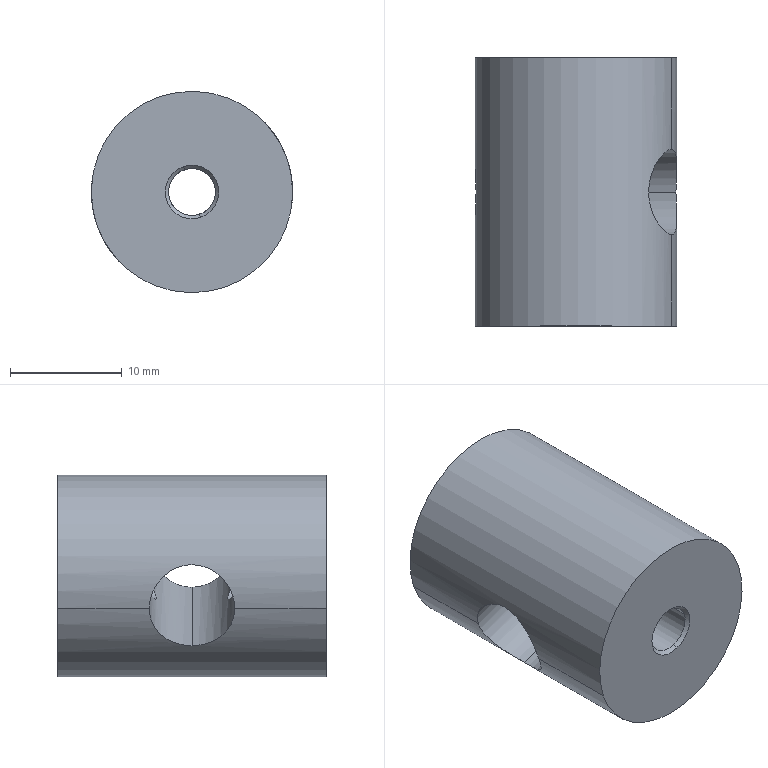Part | STEP file | 2026.6.15-Main Assembly图.sldasm-Part-182 | 1 solid | 14 faces | box 18 x 24 x 18 mm | volume 5067 mm3 | cylinder 8 | cone 4 | plane 2 | commonest cylinder face diameters 4.2 x4 7.65 x2 18 x2
STEP:
#1=CARTESIAN_POINT('',(-1463.721,1436.264,3252.695));
#2=VERTEX_POINT('',#1);
#3=CARTESIAN_POINT('',(-1463.437,1435.964,3252.791));
#4=VERTEX_POINT('',#3);
#5=CARTESIAN_POINT('',(-1463.721,1436.264,3252.695));
#6=DIRECTION('',(0.6699,-0.7071,0.2262));
#7=VECTOR('',#6,1000.);
#8=LINE('',#5,#7);
#9=EDGE_CURVE('',#2,#4,#8,.T.);
#10=ORIENTED_EDGE('',*,*,#9,.T.);
#11=CARTESIAN_POINT('',(-1459.458,1435.964,3254.134));
#12=VERTEX_POINT('',#11);
#13=CARTESIAN_POINT('',(-1461.448,1435.964,3253.462));
#14=DIRECTION('',(0.,-1.,0.));
#15=DIRECTION('',(0.9474,0.,0.3199));
#16=AXIS2_PLACEMENT_3D('',#13,#14,#15);
#17=CIRCLE('',#16,2.1);
#18=EDGE_CURVE('',#4,#12,#17,.T.);
#19=ORIENTED_EDGE('',*,*,#18,.T.);
#20=CARTESIAN_POINT('',(-1459.174,1436.264,3254.23));
#21=VERTEX_POINT('',#20);
#22=CARTESIAN_POINT('',(-1459.174,1436.264,3254.23));
#23=DIRECTION('',(-0.6699,-0.7071,-0.2262));
#24=VECTOR('',#23,1000.);
#25=LINE('',#22,#24);
#26=EDGE_CURVE('',#21,#12,#25,.T.);
#27=ORIENTED_EDGE('',*,*,#26,.F.);
#28=CARTESIAN_POINT('',(-1461.448,1436.264,3253.462));
#29=DIRECTION('',(0.,-1.,0.));
#30=DIRECTION('',(0.9474,0.,0.3199));
#31=AXIS2_PLACEMENT_3D('',#28,#29,#30);
#32=CIRCLE('',#31,2.4);
#33=EDGE_CURVE('',#2,#21,#32,.T.);
#34=ORIENTED_EDGE('',*,*,#33,.F.);
#35=EDGE_LOOP('',(#10,#19,#27,#34));
#36=FACE_OUTER_BOUND('',#35,.T.);
#37=CARTESIAN_POINT('',(-1461.448,1436.264,3253.462));
#38=DIRECTION('',(0.,1.,0.));
#39=DIRECTION('',(-0.9474,0.,-0.3199));
#40=AXIS2_PLACEMENT_3D('',#37,#38,#39);
#41=CONICAL_SURFACE('',#40,2.4,0.7854);
#42=ADVANCED_FACE('',(#36),#41,.F.);
#43=CARTESIAN_POINT('',(-1462.12,1412.564,3255.452));
#44=VERTEX_POINT('',#43);
#45=CARTESIAN_POINT('',(-1462.216,1412.264,3255.736));
#46=VERTEX_POINT('',#45);
#47=CARTESIAN_POINT('',(-1462.216,1412.264,3255.736));
#48=DIRECTION('',(-0.2262,-0.7071,0.6699));
#49=VECTOR('',#48,1000.);
#50=LINE('',#47,#49);
#51=EDGE_CURVE('',#44,#46,#50,.T.);
#52=ORIENTED_EDGE('',*,*,#51,.F.);
#53=CARTESIAN_POINT('',(-1459.458,1412.564,3254.134));
#54=VERTEX_POINT('',#53);
#55=CARTESIAN_POINT('',(-1461.448,1412.564,3253.462));
#56=DIRECTION('',(0.,1.,0.));
#57=DIRECTION('',(0.9474,0.,0.3199));
#58=AXIS2_PLACEMENT_3D('',#55,#56,#57);
#59=CIRCLE('',#58,2.1);
#60=EDGE_CURVE('',#44,#54,#59,.T.);
#61=ORIENTED_EDGE('',*,*,#60,.T.);
#62=CARTESIAN_POINT('',(-1460.776,1412.564,3251.473));
#63=VERTEX_POINT('',#62);
#64=CARTESIAN_POINT('',(-1461.448,1412.564,3253.462));
#65=DIRECTION('',(0.,1.,0.));
#66=DIRECTION('',(0.9474,0.,0.3199));
#67=AXIS2_PLACEMENT_3D('',#64,#65,#66);
#68=CIRCLE('',#67,2.1);
#69=EDGE_CURVE('',#54,#63,#68,.T.);
#70=ORIENTED_EDGE('',*,*,#69,.T.);
#71=CARTESIAN_POINT('',(-1460.68,1412.264,3251.189));
#72=VERTEX_POINT('',#71);
#73=CARTESIAN_POINT('',(-1460.68,1412.264,3251.189));
#74=DIRECTION('',(0.2262,-0.7071,-0.6699));
#75=VECTOR('',#74,1000.);
#76=LINE('',#73,#75);
#77=EDGE_CURVE('',#63,#72,#76,.T.);
#78=ORIENTED_EDGE('',*,*,#77,.T.);
#79=CARTESIAN_POINT('',(-1461.448,1412.264,3253.462));
#80=DIRECTION('',(0.,-1.,0.));
#81=DIRECTION('',(0.3199,0.,-0.9474));
#82=AXIS2_PLACEMENT_3D('',#79,#80,#81);
#83=CIRCLE('',#82,2.4);
#84=EDGE_CURVE('',#72,#46,#83,.T.);
#85=ORIENTED_EDGE('',*,*,#84,.T.);
#86=EDGE_LOOP('',(#52,#61,#70,#78,#85));
#87=FACE_OUTER_BOUND('',#86,.T.);
#88=CARTESIAN_POINT('',(-1461.448,1412.264,3253.462));
#89=DIRECTION('',(0.,-1.,0.));
#90=DIRECTION('',(-0.3199,0.,0.9474));
#91=AXIS2_PLACEMENT_3D('',#88,#89,#90);
#92=CONICAL_SURFACE('',#91,2.4,0.7854);
#93=ADVANCED_FACE('',(#87),#92,.F.);
#94=CARTESIAN_POINT('',(-1463.437,1420.439,3252.791));
#95=VERTEX_POINT('',#94);
#96=CARTESIAN_POINT('',(-1463.437,1412.564,3252.791));
#97=VERTEX_POINT('',#96);
#98=CARTESIAN_POINT('',(-1463.437,1436.264,3252.791));
#99=DIRECTION('',(0.,-1.,0.));
#100=VECTOR('',#99,1000.);
#101=LINE('',#98,#100);
#102=EDGE_CURVE('',#95,#97,#101,.T.);
#103=ORIENTED_EDGE('',*,*,#102,.T.);
#104=CARTESIAN_POINT('',(-1461.448,1412.564,3253.462));
#105=DIRECTION('',(0.,1.,0.));
#106=DIRECTION('',(0.9474,0.,0.3199));
#107=AXIS2_PLACEMENT_3D('',#104,#105,#106);
#108=CIRCLE('',#107,2.1);
#109=EDGE_CURVE('',#63,#97,#108,.T.);
#110=ORIENTED_EDGE('',*,*,#109,.F.);
#111=ORIENTED_EDGE('',*,*,#69,.F.);
#112=CARTESIAN_POINT('',(-1459.458,1420.439,3254.134));
#113=VERTEX_POINT('',#112);
#114=CARTESIAN_POINT('',(-1459.458,1436.264,3254.134));
#115=DIRECTION('',(0.,-1.,0.));
#116=VECTOR('',#115,1000.);
#117=LINE('',#114,#116);
#118=EDGE_CURVE('',#113,#54,#117,.T.);
#119=ORIENTED_EDGE('',*,*,#118,.F.);
#120=CARTESIAN_POINT('',(-1459.458,1420.439,3254.134));
#121=CARTESIAN_POINT('',(-1459.413,1420.439,3254.));
#122=CARTESIAN_POINT('',(-1459.382,1420.447,3253.864));
#123=CARTESIAN_POINT('',(-1459.347,1420.477,3253.588));
#124=CARTESIAN_POINT('',(-1459.343,1420.5,3253.447));
#125=CARTESIAN_POINT('',(-1459.373,1420.582,3253.035));
#126=CARTESIAN_POINT('',(-1459.447,1420.66,3252.769));
#127=CARTESIAN_POINT('',(-1459.626,1420.78,3252.408));
#128=CARTESIAN_POINT('',(-1459.698,1420.821,3252.293));
#129=CARTESIAN_POINT('',(-1459.863,1420.898,3252.078));
#130=CARTESIAN_POINT('',(-1459.954,1420.934,3251.98));
#131=CARTESIAN_POINT('',(-1460.158,1420.996,3251.799));
#132=CARTESIAN_POINT('',(-1460.272,1421.022,3251.717));
#133=CARTESIAN_POINT('',(-1460.512,1421.058,3251.577));
#134=CARTESIAN_POINT('',(-1460.639,1421.067,3251.519));
#135=CARTESIAN_POINT('',(-1460.904,1421.068,3251.429));
#136=CARTESIAN_POINT('',(-1461.044,1421.058,3251.397));
#137=CARTESIAN_POINT('',(-1461.319,1421.023,3251.362));
#138=CARTESIAN_POINT('',(-1461.459,1420.997,3251.358));
#139=CARTESIAN_POINT('',(-1461.87,1420.904,3251.387));
#140=CARTESIAN_POINT('',(-1462.135,1420.82,3251.46));
#141=CARTESIAN_POINT('',(-1462.617,1420.66,3251.697));
#142=CARTESIAN_POINT('',(-1462.838,1420.583,3251.865));
#143=CARTESIAN_POINT('',(-1463.11,1420.5,3252.172));
#144=CARTESIAN_POINT('',(-1463.193,1420.478,3252.286));
#145=CARTESIAN_POINT('',(-1463.334,1420.447,3252.528));
#146=CARTESIAN_POINT('',(-1463.392,1420.439,3252.656));
#147=CARTESIAN_POINT('',(-1463.437,1420.439,3252.791));
#148=B_SPLINE_CURVE_WITH_KNOTS('',3,(#120,#121,#122,#123,#124,#125,#126,#127,#128,#129,#130,#131,#132,#133,#134,#135,#136,#137,#138,#139,#140,#141,#142,#143,#144,#145,#146,#147),.UNSPECIFIED.,.F.,.F.,(4,2,2,2,2,2,2,2,2,2,2,2,2,4),(0.,0.000419,0.000838,0.001676,0.002095,0.002514,0.002933,0.003352,0.003771,0.00419,0.005028,0.005866,0.006285,0.006704),.UNSPECIFIED.);
#149=EDGE_CURVE('',#113,#95,#148,.T.);
#150=ORIENTED_EDGE('',*,*,#149,.T.);
#151=EDGE_LOOP('',(#103,#110,#111,#119,#150));
#152=FACE_OUTER_BOUND('',#151,.T.);
#153=CARTESIAN_POINT('',(-1461.448,1436.264,3253.462));
#154=DIRECTION('',(0.,1.,0.));
#155=DIRECTION('',(-0.9474,0.,-0.3199));
#156=AXIS2_PLACEMENT_3D('',#153,#154,#155);
#157=CYLINDRICAL_SURFACE('',#156,2.1);
#158=ADVANCED_FACE('',(#152),#157,.F.);
#159=CARTESIAN_POINT('',(-1463.437,1428.089,3252.791));
#160=VERTEX_POINT('',#159);
#161=CARTESIAN_POINT('',(-1463.437,1436.264,3252.791));
#162=DIRECTION('',(0.,-1.,0.));
#163=VECTOR('',#162,1000.);
#164=LINE('',#161,#163);
#165=EDGE_CURVE('',#4,#160,#164,.T.);
#166=ORIENTED_EDGE('',*,*,#165,.T.);
#167=CARTESIAN_POINT('',(-1459.458,1428.089,3254.134));
#168=VERTEX_POINT('',#167);
#169=CARTESIAN_POINT('',(-1463.437,1428.089,3252.791));
#170=CARTESIAN_POINT('',(-1463.392,1428.089,3252.656));
#171=CARTESIAN_POINT('',(-1463.334,1428.081,3252.529));
#172=CARTESIAN_POINT('',(-1463.194,1428.052,3252.289));
#173=CARTESIAN_POINT('',(-1463.112,1428.029,3252.174));
#174=CARTESIAN_POINT('',(-1462.838,1427.946,3251.865));
#175=CARTESIAN_POINT('',(-1462.618,1427.869,3251.698));
#176=CARTESIAN_POINT('',(-1462.257,1427.749,3251.52));
#177=CARTESIAN_POINT('',(-1462.13,1427.708,3251.472));
#178=CARTESIAN_POINT('',(-1461.869,1427.63,3251.401));
#179=CARTESIAN_POINT('',(-1461.736,1427.594,3251.378));
#180=CARTESIAN_POINT('',(-1461.465,1427.532,3251.358));
#181=CARTESIAN_POINT('',(-1461.324,1427.506,3251.362));
#182=CARTESIAN_POINT('',(-1461.048,1427.471,3251.396));
#183=CARTESIAN_POINT('',(-1460.913,1427.461,3251.427));
#184=CARTESIAN_POINT('',(-1460.647,1427.461,3251.516));
#185=CARTESIAN_POINT('',(-1460.517,1427.471,3251.575));
#186=CARTESIAN_POINT('',(-1460.276,1427.506,3251.714));
#187=CARTESIAN_POINT('',(-1460.163,1427.531,3251.796));
#188=CARTESIAN_POINT('',(-1459.853,1427.625,3252.068));
#189=CARTESIAN_POINT('',(-1459.687,1427.708,3252.287));
#190=CARTESIAN_POINT('',(-1459.448,1427.868,3252.768));
#191=CARTESIAN_POINT('',(-1459.374,1427.946,3253.035));
#192=CARTESIAN_POINT('',(-1459.343,1428.029,3253.444));
#193=CARTESIAN_POINT('',(-1459.347,1428.051,3253.585));
#194=CARTESIAN_POINT('',(-1459.381,1428.081,3253.863));
#195=CARTESIAN_POINT('',(-1459.413,1428.089,3254.));
#196=CARTESIAN_POINT('',(-1459.458,1428.089,3254.134));
#197=B_SPLINE_CURVE_WITH_KNOTS('',3,(#169,#170,#171,#172,#173,#174,#175,#176,#177,#178,#179,#180,#181,#182,#183,#184,#185,#186,#187,#188,#189,#190,#191,#192,#193,#194,#195,#196),.UNSPECIFIED.,.F.,.F.,(4,2,2,2,2,2,2,2,2,2,2,2,2,4),(0.,0.000419,0.000838,0.001676,0.002095,0.002514,0.002933,0.003352,0.003771,0.00419,0.005028,0.005866,0.006285,0.006704),.UNSPECIFIED.);
#198=EDGE_CURVE('',#160,#168,#197,.T.);
#199=ORIENTED_EDGE('',*,*,#198,.T.);
#200=CARTESIAN_POINT('',(-1459.458,1436.264,3254.134));
#201=DIRECTION('',(0.,-1.,0.));
#202=VECTOR('',#201,1000.);
#203=LINE('',#200,#202);
#204=EDGE_CURVE('',#12,#168,#203,.T.);
#205=ORIENTED_EDGE('',*,*,#204,.F.);
#206=ORIENTED_EDGE('',*,*,#18,.F.);
#207=EDGE_LOOP('',(#166,#199,#205,#206));
#208=FACE_OUTER_BOUND('',#207,.T.);
#209=CARTESIAN_POINT('',(-1461.448,1436.264,3253.462));
#210=DIRECTION('',(0.,1.,0.));
#211=DIRECTION('',(-0.9474,0.,-0.3199));
#212=AXIS2_PLACEMENT_3D('',#209,#210,#211);
#213=CYLINDRICAL_SURFACE('',#212,2.1);
#214=ADVANCED_FACE('',(#208),#213,.F.);
#215=CARTESIAN_POINT('',(-1469.975,1436.264,3250.583));
#216=VERTEX_POINT('',#215);
#217=CARTESIAN_POINT('',(-1452.921,1436.264,3256.342));
#218=VERTEX_POINT('',#217);
#219=CARTESIAN_POINT('',(-1461.448,1436.264,3253.462));
#220=DIRECTION('',(0.,-1.,0.));
#221=DIRECTION('',(-0.9474,0.,-0.3199));
#222=AXIS2_PLACEMENT_3D('',#219,#220,#221);
#223=CIRCLE('',#222,9.);
#224=EDGE_CURVE('',#216,#218,#223,.T.);
#225=ORIENTED_EDGE('',*,*,#224,.F.);
#226=CARTESIAN_POINT('',(-1461.448,1436.264,3253.462));
#227=DIRECTION('',(0.,-1.,0.));
#228=DIRECTION('',(-0.9474,0.,-0.3199));
#229=AXIS2_PLACEMENT_3D('',#226,#227,#228);
#230=CIRCLE('',#229,9.);
#231=EDGE_CURVE('',#218,#216,#230,.T.);
#232=ORIENTED_EDGE('',*,*,#231,.F.);
#233=EDGE_LOOP('',(#225,#232));
#234=FACE_OUTER_BOUND('',#233,.T.);
#235=CARTESIAN_POINT('',(-1461.448,1436.264,3253.462));
#236=DIRECTION('',(0.,-1.,0.));
#237=DIRECTION('',(0.9474,0.,0.3199));
#238=AXIS2_PLACEMENT_3D('',#235,#236,#237);
#239=CIRCLE('',#238,2.4);
#240=EDGE_CURVE('',#21,#2,#239,.T.);
#241=ORIENTED_EDGE('',*,*,#240,.T.);
#242=ORIENTED_EDGE('',*,*,#33,.T.);
#243=EDGE_LOOP('',(#241,#242));
#244=FACE_BOUND('',#243,.T.);
#245=CARTESIAN_POINT('',(-1461.448,1436.264,3253.462));
#246=DIRECTION('',(0.,1.,0.));
#247=DIRECTION('',(1.,0.,0.));
#248=AXIS2_PLACEMENT_3D('',#245,#246,#247);
#249=PLANE('',#248);
#250=ADVANCED_FACE('',(#234,#244),#249,.T.);
#251=CARTESIAN_POINT('',(-1469.975,1412.264,3250.583));
#252=VERTEX_POINT('',#251);
#253=CARTESIAN_POINT('',(-1452.921,1412.264,3256.342));
#254=VERTEX_POINT('',#253);
#255=CARTESIAN_POINT('',(-1461.448,1412.264,3253.462));
#256=DIRECTION('',(0.,1.,0.));
#257=DIRECTION('',(-0.9474,0.,-0.3199));
#258=AXIS2_PLACEMENT_3D('',#255,#256,#257);
#259=CIRCLE('',#258,9.);
#260=EDGE_CURVE('',#252,#254,#259,.T.);
#261=ORIENTED_EDGE('',*,*,#260,.F.);
#262=CARTESIAN_POINT('',(-1461.448,1412.264,3253.462));
#263=DIRECTION('',(0.,1.,0.));
#264=DIRECTION('',(-0.9474,0.,-0.3199));
#265=AXIS2_PLACEMENT_3D('',#262,#263,#264);
#266=CIRCLE('',#265,9.);
#267=EDGE_CURVE('',#254,#252,#266,.T.);
#268=ORIENTED_EDGE('',*,*,#267,.F.);
#269=EDGE_LOOP('',(#261,#268));
#270=FACE_OUTER_BOUND('',#269,.T.);
#271=ORIENTED_EDGE('',*,*,#84,.F.);
#272=CARTESIAN_POINT('',(-1461.448,1412.264,3253.462));
#273=DIRECTION('',(0.,-1.,0.));
#274=DIRECTION('',(0.3199,0.,-0.9474));
#275=AXIS2_PLACEMENT_3D('',#272,#273,#274);
#276=CIRCLE('',#275,2.4);
#277=EDGE_CURVE('',#46,#72,#276,.T.);
#278=ORIENTED_EDGE('',*,*,#277,.F.);
#279=EDGE_LOOP('',(#271,#278));
#280=FACE_BOUND('',#279,.T.);
#281=CARTESIAN_POINT('',(-1461.448,1412.264,3253.462));
#282=DIRECTION('',(0.,1.,0.));
#283=DIRECTION('',(1.,0.,0.));
#284=AXIS2_PLACEMENT_3D('',#281,#282,#283);
#285=PLANE('',#284);
#286=ADVANCED_FACE('',(#270,#280),#285,.F.);
#287=CARTESIAN_POINT('',(-1470.39,1424.264,3254.48));
#288=VERTEX_POINT('',#287);
#289=CARTESIAN_POINT('',(-1454.953,1424.264,3259.693));
#290=VERTEX_POINT('',#289);
#291=CARTESIAN_POINT('',(-1498.2,1424.264,3245.088));
#292=DIRECTION('',(0.9474,0.,0.3199));
#293=VECTOR('',#292,1000.);
#294=LINE('',#291,#293);
#295=EDGE_CURVE('',#288,#290,#294,.T.);
#296=ORIENTED_EDGE('',*,*,#295,.F.);
#297=CARTESIAN_POINT('',(-1469.975,1428.089,3250.583));
#298=VERTEX_POINT('',#297);
#299=CARTESIAN_POINT('',(-1469.975,1428.089,3250.583));
#300=CARTESIAN_POINT('',(-1470.056,1428.089,3250.825));
#301=CARTESIAN_POINT('',(-1470.126,1428.064,3251.067));
#302=CARTESIAN_POINT('',(-1470.245,1427.965,3251.547));
#303=CARTESIAN_POINT('',(-1470.294,1427.89,3251.789));
#304=CARTESIAN_POINT('',(-1470.369,1427.697,3252.251));
#305=CARTESIAN_POINT('',(-1470.396,1427.579,3252.472));
#306=CARTESIAN_POINT('',(-1470.432,1427.302,3252.896));
#307=CARTESIAN_POINT('',(-1470.442,1427.142,3253.097));
#308=CARTESIAN_POINT('',(-1470.449,1426.794,3253.462));
#309=CARTESIAN_POINT('',(-1470.447,1426.603,3253.629));
#310=CARTESIAN_POINT('',(-1470.437,1426.188,3253.926));
#311=CARTESIAN_POINT('',(-1470.429,1425.97,3254.053));
#312=CARTESIAN_POINT('',(-1470.413,1425.512,3254.26));
#313=CARTESIAN_POINT('',(-1470.405,1425.268,3254.343));
#314=CARTESIAN_POINT('',(-1470.393,1424.772,3254.452));
#315=CARTESIAN_POINT('',(-1470.39,1424.52,3254.48));
#316=CARTESIAN_POINT('',(-1470.39,1424.264,3254.48));
#317=B_SPLINE_CURVE_WITH_KNOTS('',3,(#299,#300,#301,#302,#303,#304,#305,#306,#307,#308,#309,#310,#311,#312,#313,#314,#315,#316),.UNSPECIFIED.,.F.,.F.,(4,2,2,2,2,2,2,2,4),(0.,0.0007561,0.001512,0.002268,0.003024,0.003781,0.004537,0.005293,0.006049),.UNSPECIFIED.);
#318=EDGE_CURVE('',#298,#288,#317,.T.);
#319=ORIENTED_EDGE('',*,*,#318,.F.);
#320=CARTESIAN_POINT('',(-1467.942,1424.264,3247.232));
#321=VERTEX_POINT('',#320);
#322=CARTESIAN_POINT('',(-1467.942,1424.264,3247.232));
#323=CARTESIAN_POINT('',(-1467.942,1424.52,3247.232));
#324=CARTESIAN_POINT('',(-1467.962,1424.771,3247.252));
#325=CARTESIAN_POINT('',(-1468.037,1425.264,3247.331));
#326=CARTESIAN_POINT('',(-1468.093,1425.508,3247.392));
#327=CARTESIAN_POINT('',(-1468.232,1425.969,3247.548));
#328=CARTESIAN_POINT('',(-1468.315,1426.188,3247.644));
#329=CARTESIAN_POINT('',(-1468.503,1426.601,3247.873));
#330=CARTESIAN_POINT('',(-1468.607,1426.794,3248.005));
#331=CARTESIAN_POINT('',(-1468.822,1427.142,3248.3));
#332=CARTESIAN_POINT('',(-1468.935,1427.3,3248.464));
#333=CARTESIAN_POINT('',(-1469.163,1427.579,3248.824));
#334=CARTESIAN_POINT('',(-1469.276,1427.696,3249.017));
#335=CARTESIAN_POINT('',(-1469.496,1427.889,3249.427));
#336=CARTESIAN_POINT('',(-1469.603,1427.964,3249.648));
#337=CARTESIAN_POINT('',(-1469.802,1428.064,3250.105));
#338=CARTESIAN_POINT('',(-1469.893,1428.089,3250.341));
#339=CARTESIAN_POINT('',(-1469.975,1428.089,3250.583));
#340=B_SPLINE_CURVE_WITH_KNOTS('',3,(#322,#323,#324,#325,#326,#327,#328,#329,#330,#331,#332,#333,#334,#335,#336,#337,#338,#339),.UNSPECIFIED.,.F.,.F.,(4,2,2,2,2,2,2,2,4),(0.,0.000756,0.001512,0.002268,0.003024,0.00378,0.004536,0.005292,0.006048),.UNSPECIFIED.);
#341=EDGE_CURVE('',#321,#298,#340,.T.);
#342=ORIENTED_EDGE('',*,*,#341,.F.);
#343=CARTESIAN_POINT('',(-1452.505,1424.264,3252.445));
#344=VERTEX_POINT('',#343);
#345=CARTESIAN_POINT('',(-1495.753,1424.264,3237.841));
#346=DIRECTION('',(0.9474,0.,0.3199));
#347=VECTOR('',#346,1000.);
#348=LINE('',#345,#347);
#349=EDGE_CURVE('',#321,#344,#348,.T.);
#350=ORIENTED_EDGE('',*,*,#349,.T.);
#351=CARTESIAN_POINT('',(-1452.921,1428.089,3256.342));
#352=VERTEX_POINT('',#351);
#353=CARTESIAN_POINT('',(-1452.921,1428.089,3256.342));
#354=CARTESIAN_POINT('',(-1452.839,1428.089,3256.1));
#355=CARTESIAN_POINT('',(-1452.769,1428.064,3255.858));
#356=CARTESIAN_POINT('',(-1452.65,1427.965,3255.378));
#357=CARTESIAN_POINT('',(-1452.602,1427.89,3255.136));
#358=CARTESIAN_POINT('',(-1452.526,1427.697,3254.674));
#359=CARTESIAN_POINT('',(-1452.5,1427.579,3254.452));
#360=CARTESIAN_POINT('',(-1452.463,1427.302,3254.028));
#361=CARTESIAN_POINT('',(-1452.453,1427.142,3253.828));
#362=CARTESIAN_POINT('',(-1452.446,1426.794,3253.463));
#363=CARTESIAN_POINT('',(-1452.448,1426.603,3253.296));
#364=CARTESIAN_POINT('',(-1452.458,1426.188,3252.999));
#365=CARTESIAN_POINT('',(-1452.466,1425.97,3252.872));
#366=CARTESIAN_POINT('',(-1452.482,1425.512,3252.664));
#367=CARTESIAN_POINT('',(-1452.491,1425.268,3252.582));
#368=CARTESIAN_POINT('',(-1452.502,1424.772,3252.473));
#369=CARTESIAN_POINT('',(-1452.505,1424.52,3252.445));
#370=CARTESIAN_POINT('',(-1452.505,1424.264,3252.445));
#371=B_SPLINE_CURVE_WITH_KNOTS('',3,(#353,#354,#355,#356,#357,#358,#359,#360,#361,#362,#363,#364,#365,#366,#367,#368,#369,#370),.UNSPECIFIED.,.F.,.F.,(4,2,2,2,2,2,2,2,4),(0.,0.0007561,0.001512,0.002268,0.003024,0.003781,0.004537,0.005293,0.006049),.UNSPECIFIED.);
#372=EDGE_CURVE('',#352,#344,#371,.T.);
#373=ORIENTED_EDGE('',*,*,#372,.F.);
#374=CARTESIAN_POINT('',(-1454.953,1424.264,3259.693));
#375=CARTESIAN_POINT('',(-1454.953,1424.52,3259.693));
#376=CARTESIAN_POINT('',(-1454.933,1424.771,3259.673));
#377=CARTESIAN_POINT('',(-1454.859,1425.264,3259.593));
#378=CARTESIAN_POINT('',(-1454.803,1425.508,3259.533));
#379=CARTESIAN_POINT('',(-1454.663,1425.969,3259.377));
#380=CARTESIAN_POINT('',(-1454.58,1426.188,3259.281));
#381=CARTESIAN_POINT('',(-1454.392,1426.601,3259.052));
#382=CARTESIAN_POINT('',(-1454.289,1426.794,3258.92));
#383=CARTESIAN_POINT('',(-1454.073,1427.142,3258.625));
#384=CARTESIAN_POINT('',(-1453.96,1427.3,3258.461));
#385=CARTESIAN_POINT('',(-1453.732,1427.579,3258.1));
#386=CARTESIAN_POINT('',(-1453.619,1427.696,3257.908));
#387=CARTESIAN_POINT('',(-1453.4,1427.889,3257.498));
#388=CARTESIAN_POINT('',(-1453.292,1427.964,3257.277));
#389=CARTESIAN_POINT('',(-1453.094,1428.064,3256.82));
#390=CARTESIAN_POINT('',(-1453.003,1428.089,3256.584));
#391=CARTESIAN_POINT('',(-1452.921,1428.089,3256.342));
#392=B_SPLINE_CURVE_WITH_KNOTS('',3,(#374,#375,#376,#377,#378,#379,#380,#381,#382,#383,#384,#385,#386,#387,#388,#389,#390,#391),.UNSPECIFIED.,.F.,.F.,(4,2,2,2,2,2,2,2,4),(0.,0.000756,0.001512,0.002268,0.003024,0.00378,0.004536,0.005292,0.006048),.UNSPECIFIED.);
#393=EDGE_CURVE('',#290,#352,#392,.T.);
#394=ORIENTED_EDGE('',*,*,#393,.F.);
#395=EDGE_LOOP('',(#296,#319,#342,#350,#373,#394));
#396=FACE_OUTER_BOUND('',#395,.T.);
#397=CARTESIAN_POINT('',(-1459.458,1428.089,3254.134));
#398=CARTESIAN_POINT('',(-1459.503,1428.089,3254.269));
#399=CARTESIAN_POINT('',(-1459.561,1428.081,3254.396));
#400=CARTESIAN_POINT('',(-1459.701,1428.052,3254.636));
#401=CARTESIAN_POINT('',(-1459.784,1428.029,3254.751));
#402=CARTESIAN_POINT('',(-1460.057,1427.946,3255.06));
#403=CARTESIAN_POINT('',(-1460.277,1427.869,3255.227));
#404=CARTESIAN_POINT('',(-1460.638,1427.749,3255.405));
#405=CARTESIAN_POINT('',(-1460.765,1427.708,3255.453));
#406=CARTESIAN_POINT('',(-1461.026,1427.63,3255.524));
#407=CARTESIAN_POINT('',(-1461.159,1427.594,3255.547));
#408=CARTESIAN_POINT('',(-1461.431,1427.532,3255.567));
#409=CARTESIAN_POINT('',(-1461.572,1427.506,3255.563));
#410=CARTESIAN_POINT('',(-1461.847,1427.471,3255.529));
#411=CARTESIAN_POINT('',(-1461.982,1427.461,3255.498));
#412=CARTESIAN_POINT('',(-1462.248,1427.461,3255.409));
#413=CARTESIAN_POINT('',(-1462.378,1427.471,3255.35));
#414=CARTESIAN_POINT('',(-1462.619,1427.506,3255.211));
#415=CARTESIAN_POINT('',(-1462.733,1427.531,3255.129));
#416=CARTESIAN_POINT('',(-1463.042,1427.625,3254.857));
#417=CARTESIAN_POINT('',(-1463.208,1427.708,3254.638));
#418=CARTESIAN_POINT('',(-1463.447,1427.868,3254.157));
#419=CARTESIAN_POINT('',(-1463.522,1427.946,3253.89));
#420=CARTESIAN_POINT('',(-1463.552,1428.029,3253.481));
#421=CARTESIAN_POINT('',(-1463.549,1428.051,3253.34));
#422=CARTESIAN_POINT('',(-1463.514,1428.081,3253.062));
#423=CARTESIAN_POINT('',(-1463.483,1428.089,3252.925));
#424=CARTESIAN_POINT('',(-1463.437,1428.089,3252.791));
#425=B_SPLINE_CURVE_WITH_KNOTS('',3,(#397,#398,#399,#400,#401,#402,#403,#404,#405,#406,#407,#408,#409,#410,#411,#412,#413,#414,#415,#416,#417,#418,#419,#420,#421,#422,#423,#424),.UNSPECIFIED.,.F.,.F.,(4,2,2,2,2,2,2,2,2,2,2,2,2,4),(0.,0.000419,0.000838,0.001676,0.002095,0.002514,0.002933,0.003352,0.003771,0.00419,0.005028,0.005866,0.006285,0.006704),.UNSPECIFIED.);
#426=EDGE_CURVE('',#168,#160,#425,.T.);
#427=ORIENTED_EDGE('',*,*,#426,.F.);
#428=ORIENTED_EDGE('',*,*,#198,.F.);
#429=EDGE_LOOP('',(#427,#428));
#430=FACE_BOUND('',#429,.T.);
#431=CARTESIAN_POINT('',(-1496.977,1424.264,3241.465));
#432=DIRECTION('',(0.9474,0.,0.3199));
#433=DIRECTION('',(-0.3199,0.,0.9474));
#434=AXIS2_PLACEMENT_3D('',#431,#432,#433);
#435=CYLINDRICAL_SURFACE('',#434,3.825);
#436=ADVANCED_FACE('',(#396,#430),#435,.F.);
#437=CARTESIAN_POINT('',(-1452.921,1436.264,3256.342));
#438=DIRECTION('',(0.,-1.,0.));
#439=VECTOR('',#438,1000.);
#440=LINE('',#437,#439);
#441=EDGE_CURVE('',#218,#352,#440,.T.);
#442=ORIENTED_EDGE('',*,*,#441,.F.);
#443=ORIENTED_EDGE('',*,*,#231,.T.);
#444=CARTESIAN_POINT('',(-1469.975,1436.264,3250.583));
#445=DIRECTION('',(0.,-1.,0.));
#446=VECTOR('',#445,1000.);
#447=LINE('',#444,#446);
#448=EDGE_CURVE('',#216,#298,#447,.T.);
#449=ORIENTED_EDGE('',*,*,#448,.T.);
#450=ORIENTED_EDGE('',*,*,#318,.T.);
#451=CARTESIAN_POINT('',(-1469.975,1420.439,3250.583));
#452=VERTEX_POINT('',#451);
#453=CARTESIAN_POINT('',(-1470.39,1424.264,3254.48));
#454=CARTESIAN_POINT('',(-1470.39,1424.008,3254.48));
#455=CARTESIAN_POINT('',(-1470.393,1423.757,3254.452));
#456=CARTESIAN_POINT('',(-1470.405,1423.265,3254.344));
#457=CARTESIAN_POINT('',(-1470.413,1423.021,3254.262));
#458=CARTESIAN_POINT('',(-1470.429,1422.559,3254.053));
#459=CARTESIAN_POINT('',(-1470.437,1422.341,3253.926));
#460=CARTESIAN_POINT('',(-1470.447,1421.928,3253.631));
#461=CARTESIAN_POINT('',(-1470.449,1421.735,3253.462));
#462=CARTESIAN_POINT('',(-1470.442,1421.387,3253.097));
#463=CARTESIAN_POINT('',(-1470.432,1421.229,3252.898));
#464=CARTESIAN_POINT('',(-1470.396,1420.95,3252.473));
#465=CARTESIAN_POINT('',(-1470.369,1420.832,3252.252));
#466=CARTESIAN_POINT('',(-1470.294,1420.64,3251.792));
#467=CARTESIAN_POINT('',(-1470.246,1420.565,3251.551));
#468=CARTESIAN_POINT('',(-1470.127,1420.465,3251.068));
#469=CARTESIAN_POINT('',(-1470.056,1420.439,3250.825));
#470=CARTESIAN_POINT('',(-1469.975,1420.439,3250.583));
#471=B_SPLINE_CURVE_WITH_KNOTS('',3,(#453,#454,#455,#456,#457,#458,#459,#460,#461,#462,#463,#464,#465,#466,#467,#468,#469,#470),.UNSPECIFIED.,.F.,.F.,(4,2,2,2,2,2,2,2,4),(0.,0.000756,0.001512,0.002268,0.003024,0.00378,0.004536,0.005292,0.006048),.UNSPECIFIED.);
#472=EDGE_CURVE('',#288,#452,#471,.T.);
#473=ORIENTED_EDGE('',*,*,#472,.T.);
#474=CARTESIAN_POINT('',(-1469.975,1436.264,3250.583));
#475=DIRECTION('',(0.,-1.,0.));
#476=VECTOR('',#475,1000.);
#477=LINE('',#474,#476);
#478=EDGE_CURVE('',#452,#252,#477,.T.);
#479=ORIENTED_EDGE('',*,*,#478,.T.);
#480=ORIENTED_EDGE('',*,*,#260,.T.);
#481=CARTESIAN_POINT('',(-1452.921,1420.439,3256.342));
#482=VERTEX_POINT('',#481);
#483=CARTESIAN_POINT('',(-1452.921,1436.264,3256.342));
#484=DIRECTION('',(0.,-1.,0.));
#485=VECTOR('',#484,1000.);
#486=LINE('',#483,#485);
#487=EDGE_CURVE('',#482,#254,#486,.T.);
#488=ORIENTED_EDGE('',*,*,#487,.F.);
#489=CARTESIAN_POINT('',(-1452.921,1420.439,3256.342));
#490=CARTESIAN_POINT('',(-1453.003,1420.439,3256.584));
#491=CARTESIAN_POINT('',(-1453.093,1420.465,3256.819));
#492=CARTESIAN_POINT('',(-1453.29,1420.564,3257.273));
#493=CARTESIAN_POINT('',(-1453.398,1420.639,3257.494));
#494=CARTESIAN_POINT('',(-1453.618,1420.832,3257.907));
#495=CARTESIAN_POINT('',(-1453.731,1420.95,3258.1));
#496=CARTESIAN_POINT('',(-1453.959,1421.227,3258.459));
#497=CARTESIAN_POINT('',(-1454.073,1421.386,3258.625));
#498=CARTESIAN_POINT('',(-1454.288,1421.735,3258.919));
#499=CARTESIAN_POINT('',(-1454.392,1421.926,3259.051));
#500=CARTESIAN_POINT('',(-1454.58,1422.34,3259.281));
#501=CARTESIAN_POINT('',(-1454.663,1422.559,3259.377));
#502=CARTESIAN_POINT('',(-1454.802,1423.017,3259.532));
#503=CARTESIAN_POINT('',(-1454.858,1423.26,3259.593));
#504=CARTESIAN_POINT('',(-1454.933,1423.756,3259.673));
#505=CARTESIAN_POINT('',(-1454.953,1424.008,3259.693));
#506=CARTESIAN_POINT('',(-1454.953,1424.264,3259.693));
#507=B_SPLINE_CURVE_WITH_KNOTS('',3,(#489,#490,#491,#492,#493,#494,#495,#496,#497,#498,#499,#500,#501,#502,#503,#504,#505,#506),.UNSPECIFIED.,.F.,.F.,(4,2,2,2,2,2,2,2,4),(0.,0.0007561,0.001512,0.002268,0.003024,0.003781,0.004537,0.005293,0.006049),.UNSPECIFIED.);
#508=EDGE_CURVE('',#482,#290,#507,.T.);
#509=ORIENTED_EDGE('',*,*,#508,.T.);
#510=ORIENTED_EDGE('',*,*,#393,.T.);
#511=EDGE_LOOP('',(#442,#443,#449,#450,#473,#479,#480,#488,#509,#510));
#512=FACE_OUTER_BOUND('',#511,.T.);
#513=CARTESIAN_POINT('',(-1461.448,1436.264,3253.462));
#514=DIRECTION('',(0.,-1.,0.));
#515=DIRECTION('',(0.9474,0.,0.3199));
#516=AXIS2_PLACEMENT_3D('',#513,#514,#515);
#517=CYLINDRICAL_SURFACE('',#516,9.);
#518=ADVANCED_FACE('',(#512),#517,.T.);
#519=CARTESIAN_POINT('',(-1461.448,1435.964,3253.462));
#520=DIRECTION('',(0.,-1.,0.));
#521=DIRECTION('',(0.9474,0.,0.3199));
#522=AXIS2_PLACEMENT_3D('',#519,#520,#521);
#523=CIRCLE('',#522,2.1);
#524=EDGE_CURVE('',#12,#4,#523,.T.);
#525=ORIENTED_EDGE('',*,*,#524,.T.);
#526=ORIENTED_EDGE('',*,*,#9,.F.);
#527=ORIENTED_EDGE('',*,*,#240,.F.);
#528=ORIENTED_EDGE('',*,*,#26,.T.);
#529=EDGE_LOOP('',(#525,#526,#527,#528));
#530=FACE_OUTER_BOUND('',#529,.T.);
#531=CARTESIAN_POINT('',(-1461.448,1436.264,3253.462));
#532=DIRECTION('',(0.,1.,0.));
#533=DIRECTION('',(-0.9474,0.,-0.3199));
#534=AXIS2_PLACEMENT_3D('',#531,#532,#533);
#535=CONICAL_SURFACE('',#534,2.4,0.7854);
#536=ADVANCED_FACE('',(#530),#535,.F.);
#537=ORIENTED_EDGE('',*,*,#109,.T.);
#538=CARTESIAN_POINT('',(-1461.448,1412.564,3253.462));
#539=DIRECTION('',(0.,1.,0.));
#540=DIRECTION('',(0.9474,0.,0.3199));
#541=AXIS2_PLACEMENT_3D('',#538,#539,#540);
#542=CIRCLE('',#541,2.1);
#543=EDGE_CURVE('',#97,#44,#542,.T.);
#544=ORIENTED_EDGE('',*,*,#543,.T.);
#545=ORIENTED_EDGE('',*,*,#51,.T.);
#546=ORIENTED_EDGE('',*,*,#277,.T.);
#547=ORIENTED_EDGE('',*,*,#77,.F.);
#548=EDGE_LOOP('',(#537,#544,#545,#546,#547));
#549=FACE_OUTER_BOUND('',#548,.T.);
#550=CARTESIAN_POINT('',(-1461.448,1412.264,3253.462));
#551=DIRECTION('',(0.,-1.,0.));
#552=DIRECTION('',(-0.3199,0.,0.9474));
#553=AXIS2_PLACEMENT_3D('',#550,#551,#552);
#554=CONICAL_SURFACE('',#553,2.4,0.7854);
#555=ADVANCED_FACE('',(#549),#554,.F.);
#556=ORIENTED_EDGE('',*,*,#543,.F.);
#557=ORIENTED_EDGE('',*,*,#102,.F.);
#558=CARTESIAN_POINT('',(-1463.437,1420.439,3252.791));
#559=CARTESIAN_POINT('',(-1463.483,1420.439,3252.925));
#560=CARTESIAN_POINT('',(-1463.514,1420.447,3253.061));
#561=CARTESIAN_POINT('',(-1463.548,1420.477,3253.337));
#562=CARTESIAN_POINT('',(-1463.552,1420.5,3253.478));
#563=CARTESIAN_POINT('',(-1463.522,1420.582,3253.89));
#564=CARTESIAN_POINT('',(-1463.448,1420.66,3254.156));
#565=CARTESIAN_POINT('',(-1463.269,1420.78,3254.516));
#566=CARTESIAN_POINT('',(-1463.197,1420.821,3254.632));
#567=CARTESIAN_POINT('',(-1463.033,1420.898,3254.847));
#568=CARTESIAN_POINT('',(-1462.941,1420.934,3254.945));
#569=CARTESIAN_POINT('',(-1462.737,1420.996,3255.126));
#570=CARTESIAN_POINT('',(-1462.623,1421.022,3255.208));
#571=CARTESIAN_POINT('',(-1462.383,1421.058,3255.348));
#572=CARTESIAN_POINT('',(-1462.257,1421.067,3255.405));
#573=CARTESIAN_POINT('',(-1461.991,1421.068,3255.496));
#574=CARTESIAN_POINT('',(-1461.852,1421.058,3255.528));
#575=CARTESIAN_POINT('',(-1461.576,1421.023,3255.563));
#576=CARTESIAN_POINT('',(-1461.436,1420.997,3255.567));
#577=CARTESIAN_POINT('',(-1461.025,1420.904,3255.538));
#578=CARTESIAN_POINT('',(-1460.76,1420.82,3255.465));
#579=CARTESIAN_POINT('',(-1460.278,1420.66,3255.227));
#580=CARTESIAN_POINT('',(-1460.057,1420.583,3255.06));
#581=CARTESIAN_POINT('',(-1459.785,1420.5,3254.753));
#582=CARTESIAN_POINT('',(-1459.703,1420.478,3254.639));
#583=CARTESIAN_POINT('',(-1459.562,1420.447,3254.397));
#584=CARTESIAN_POINT('',(-1459.503,1420.439,3254.269));
#585=CARTESIAN_POINT('',(-1459.458,1420.439,3254.134));
#586=B_SPLINE_CURVE_WITH_KNOTS('',3,(#558,#559,#560,#561,#562,#563,#564,#565,#566,#567,#568,#569,#570,#571,#572,#573,#574,#575,#576,#577,#578,#579,#580,#581,#582,#583,#584,#585),.UNSPECIFIED.,.F.,.F.,(4,2,2,2,2,2,2,2,2,2,2,2,2,4),(0.,0.000419,0.000838,0.001676,0.002095,0.002514,0.002933,0.003352,0.003771,0.00419,0.005028,0.005866,0.006285,0.006704),.UNSPECIFIED.);
#587=EDGE_CURVE('',#95,#113,#586,.T.);
#588=ORIENTED_EDGE('',*,*,#587,.T.);
#589=ORIENTED_EDGE('',*,*,#118,.T.);
#590=ORIENTED_EDGE('',*,*,#60,.F.);
#591=EDGE_LOOP('',(#556,#557,#588,#589,#590));
#592=FACE_OUTER_BOUND('',#591,.T.);
#593=CARTESIAN_POINT('',(-1461.448,1436.264,3253.462));
#594=DIRECTION('',(0.,1.,0.));
#595=DIRECTION('',(-0.9474,0.,-0.3199));
#596=AXIS2_PLACEMENT_3D('',#593,#594,#595);
#597=CYLINDRICAL_SURFACE('',#596,2.1);
#598=ADVANCED_FACE('',(#592),#597,.F.);
#599=ORIENTED_EDGE('',*,*,#426,.T.);
#600=ORIENTED_EDGE('',*,*,#165,.F.);
#601=ORIENTED_EDGE('',*,*,#524,.F.);
#602=ORIENTED_EDGE('',*,*,#204,.T.);
#603=EDGE_LOOP('',(#599,#600,#601,#602));
#604=FACE_OUTER_BOUND('',#603,.T.);
#605=CARTESIAN_POINT('',(-1461.448,1436.264,3253.462));
#606=DIRECTION('',(0.,1.,0.));
#607=DIRECTION('',(-0.9474,0.,-0.3199));
#608=AXIS2_PLACEMENT_3D('',#605,#606,#607);
#609=CYLINDRICAL_SURFACE('',#608,2.1);
#610=ADVANCED_FACE('',(#604),#609,.F.);
#611=ORIENTED_EDGE('',*,*,#472,.F.);
#612=ORIENTED_EDGE('',*,*,#295,.T.);
#613=ORIENTED_EDGE('',*,*,#508,.F.);
#614=CARTESIAN_POINT('',(-1452.505,1424.264,3252.445));
#615=CARTESIAN_POINT('',(-1452.505,1424.008,3252.445));
#616=CARTESIAN_POINT('',(-1452.502,1423.757,3252.473));
#617=CARTESIAN_POINT('',(-1452.491,1423.265,3252.581));
#618=CARTESIAN_POINT('',(-1452.483,1423.021,3252.663));
#619=CARTESIAN_POINT('',(-1452.466,1422.559,3252.872));
#620=CARTESIAN_POINT('',(-1452.458,1422.341,3252.998));
#621=CARTESIAN_POINT('',(-1452.448,1421.928,3253.294));
#622=CARTESIAN_POINT('',(-1452.446,1421.735,3253.463));
#623=CARTESIAN_POINT('',(-1452.453,1421.387,3253.827));
#624=CARTESIAN_POINT('',(-1452.463,1421.229,3254.026));
#625=CARTESIAN_POINT('',(-1452.5,1420.95,3254.452));
#626=CARTESIAN_POINT('',(-1452.526,1420.832,3254.673));
#627=CARTESIAN_POINT('',(-1452.601,1420.64,3255.133));
#628=CARTESIAN_POINT('',(-1452.649,1420.565,3255.374));
#629=CARTESIAN_POINT('',(-1452.769,1420.465,3255.857));
#630=CARTESIAN_POINT('',(-1452.839,1420.439,3256.099));
#631=CARTESIAN_POINT('',(-1452.921,1420.439,3256.342));
#632=B_SPLINE_CURVE_WITH_KNOTS('',3,(#614,#615,#616,#617,#618,#619,#620,#621,#622,#623,#624,#625,#626,#627,#628,#629,#630,#631),.UNSPECIFIED.,.F.,.F.,(4,2,2,2,2,2,2,2,4),(0.,0.000756,0.001512,0.002268,0.003024,0.00378,0.004536,0.005292,0.006048),.UNSPECIFIED.);
#633=EDGE_CURVE('',#344,#482,#632,.T.);
#634=ORIENTED_EDGE('',*,*,#633,.F.);
#635=ORIENTED_EDGE('',*,*,#349,.F.);
#636=CARTESIAN_POINT('',(-1469.975,1420.439,3250.583));
#637=CARTESIAN_POINT('',(-1469.893,1420.439,3250.341));
#638=CARTESIAN_POINT('',(-1469.802,1420.465,3250.106));
#639=CARTESIAN_POINT('',(-1469.605,1420.564,3249.652));
#640=CARTESIAN_POINT('',(-1469.497,1420.639,3249.431));
#641=CARTESIAN_POINT('',(-1469.277,1420.832,3249.018));
#642=CARTESIAN_POINT('',(-1469.164,1420.95,3248.825));
#643=CARTESIAN_POINT('',(-1468.936,1421.227,3248.466));
#644=CARTESIAN_POINT('',(-1468.822,1421.386,3248.3));
#645=CARTESIAN_POINT('',(-1468.607,1421.735,3248.005));
#646=CARTESIAN_POINT('',(-1468.504,1421.926,3247.874));
#647=CARTESIAN_POINT('',(-1468.315,1422.34,3247.644));
#648=CARTESIAN_POINT('',(-1468.232,1422.559,3247.548));
#649=CARTESIAN_POINT('',(-1468.094,1423.017,3247.393));
#650=CARTESIAN_POINT('',(-1468.037,1423.26,3247.332));
#651=CARTESIAN_POINT('',(-1467.962,1423.756,3247.252));
#652=CARTESIAN_POINT('',(-1467.942,1424.008,3247.232));
#653=CARTESIAN_POINT('',(-1467.942,1424.264,3247.232));
#654=B_SPLINE_CURVE_WITH_KNOTS('',3,(#636,#637,#638,#639,#640,#641,#642,#643,#644,#645,#646,#647,#648,#649,#650,#651,#652,#653),.UNSPECIFIED.,.F.,.F.,(4,2,2,2,2,2,2,2,4),(0.,0.0007561,0.001512,0.002268,0.003024,0.003781,0.004537,0.005293,0.006049),.UNSPECIFIED.);
#655=EDGE_CURVE('',#452,#321,#654,.T.);
#656=ORIENTED_EDGE('',*,*,#655,.F.);
#657=EDGE_LOOP('',(#611,#612,#613,#634,#635,#656));
#658=FACE_OUTER_BOUND('',#657,.T.);
#659=ORIENTED_EDGE('',*,*,#149,.F.);
#660=ORIENTED_EDGE('',*,*,#587,.F.);
#661=EDGE_LOOP('',(#659,#660));
#662=FACE_BOUND('',#661,.T.);
#663=CARTESIAN_POINT('',(-1496.977,1424.264,3241.465));
#664=DIRECTION('',(0.9474,0.,0.3199));
#665=DIRECTION('',(-0.3199,0.,0.9474));
#666=AXIS2_PLACEMENT_3D('',#663,#664,#665);
#667=CYLINDRICAL_SURFACE('',#666,3.825);
#668=ADVANCED_FACE('',(#658,#662),#667,.F.);
#669=ORIENTED_EDGE('',*,*,#224,.T.);
#670=ORIENTED_EDGE('',*,*,#441,.T.);
#671=ORIENTED_EDGE('',*,*,#372,.T.);
#672=ORIENTED_EDGE('',*,*,#633,.T.);
#673=ORIENTED_EDGE('',*,*,#487,.T.);
#674=ORIENTED_EDGE('',*,*,#267,.T.);
#675=ORIENTED_EDGE('',*,*,#478,.F.);
#676=ORIENTED_EDGE('',*,*,#655,.T.);
#677=ORIENTED_EDGE('',*,*,#341,.T.);
#678=ORIENTED_EDGE('',*,*,#448,.F.);
#679=EDGE_LOOP('',(#669,#670,#671,#672,#673,#674,#675,#676,#677,#678));
#680=FACE_OUTER_BOUND('',#679,.T.);
#681=CARTESIAN_POINT('',(-1461.448,1436.264,3253.462));
#682=DIRECTION('',(0.,-1.,0.));
#683=DIRECTION('',(0.9474,0.,0.3199));
#684=AXIS2_PLACEMENT_3D('',#681,#682,#683);
#685=CYLINDRICAL_SURFACE('',#684,9.);
#686=ADVANCED_FACE('',(#680),#685,.T.);
#687=CLOSED_SHELL('',(#42,#93,#158,#214,#250,#286,#436,#518,#536,#555,#598,#610,#668,#686));
#688=MANIFOLD_SOLID_BREP('',#687);
#689=CARTESIAN_POINT('',(0.,0.,0.));
#690=DIRECTION('',(0.,0.,1.));
#691=DIRECTION('',(1.,0.,0.));
#692=AXIS2_PLACEMENT_3D('',#689,#690,#691);
#693=(LENGTH_UNIT()NAMED_UNIT(*)SI_UNIT(.MILLI.,.METRE.));
#694=UNCERTAINTY_MEASURE_WITH_UNIT(LENGTH_MEASURE(0.00001),#693,'','');
#695=(NAMED_UNIT(*)PLANE_ANGLE_UNIT()SI_UNIT($,.RADIAN.));
#696=(NAMED_UNIT(*)SI_UNIT($,.STERADIAN.)SOLID_ANGLE_UNIT());
#697=(GEOMETRIC_REPRESENTATION_CONTEXT(3)GLOBAL_UNCERTAINTY_ASSIGNED_CONTEXT((#694))GLOBAL_UNIT_ASSIGNED_CONTEXT((#693,#695,#696))REPRESENTATION_CONTEXT('',''));
#698=ADVANCED_BREP_SHAPE_REPRESENTATION('',(#688,#692),#697);